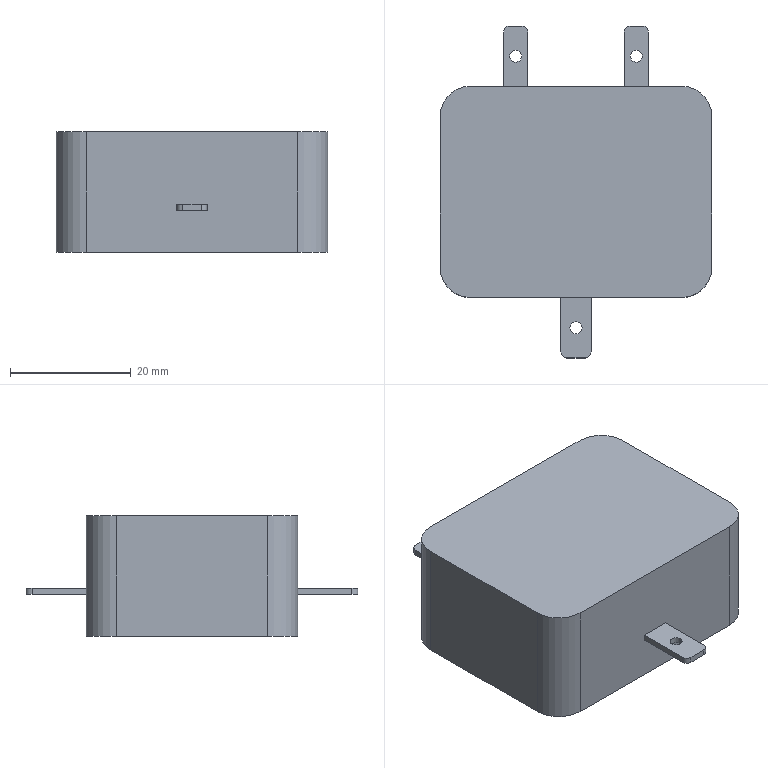Part | SolidWorks | features ICE 2, Extrusion 1 | 1 solid | 37 faces | box 45 x 55 x 20 mm | volume 31190 mm3 | plane 21 | cylinder 16 | commonest cylinder face diameters 2 x12 10 x4
STEP:
#1=CARTESIAN_POINT('',(11.,22.5,-2.));
#2=VERTEX_POINT('',#1);
#3=CARTESIAN_POINT('',(9.,22.5,-2.));
#4=VERTEX_POINT('',#3);
#5=CARTESIAN_POINT('',(10.,22.5,-2.));
#6=DIRECTION('',(0.,0.,-1.));
#7=DIRECTION('',(-1.,0.,0.));
#8=AXIS2_PLACEMENT_3D('',#5,#6,#7);
#9=CIRCLE('',#8,1.);
#10=EDGE_CURVE('',#2,#4,#9,.T.);
#11=ORIENTED_EDGE('',*,*,#10,.F.);
#12=CARTESIAN_POINT('',(11.,22.5,-3.));
#13=VERTEX_POINT('',#12);
#14=CARTESIAN_POINT('',(11.,22.5,-2.));
#15=DIRECTION('',(0.,0.,-1.));
#16=VECTOR('',#15,1000.);
#17=LINE('',#14,#16);
#18=EDGE_CURVE('',#2,#13,#17,.T.);
#19=ORIENTED_EDGE('',*,*,#18,.T.);
#20=CARTESIAN_POINT('',(9.,22.5,-3.));
#21=VERTEX_POINT('',#20);
#22=CARTESIAN_POINT('',(10.,22.5,-3.));
#23=DIRECTION('',(0.,0.,-1.));
#24=DIRECTION('',(-1.,0.,0.));
#25=AXIS2_PLACEMENT_3D('',#22,#23,#24);
#26=CIRCLE('',#25,1.);
#27=EDGE_CURVE('',#13,#21,#26,.T.);
#28=ORIENTED_EDGE('',*,*,#27,.T.);
#29=CARTESIAN_POINT('',(9.,22.5,-2.));
#30=DIRECTION('',(0.,0.,-1.));
#31=VECTOR('',#30,1000.);
#32=LINE('',#29,#31);
#33=EDGE_CURVE('',#4,#21,#32,.T.);
#34=ORIENTED_EDGE('',*,*,#33,.F.);
#35=EDGE_LOOP('',(#11,#19,#28,#34));
#36=FACE_OUTER_BOUND('',#35,.T.);
#37=CARTESIAN_POINT('',(10.,22.5,-2.));
#38=DIRECTION('',(0.,0.,-1.));
#39=DIRECTION('',(-1.,0.,0.));
#40=AXIS2_PLACEMENT_3D('',#37,#38,#39);
#41=CYLINDRICAL_SURFACE('',#40,1.);
#42=ADVANCED_FACE('',(#36),#41,.F.);
#43=CARTESIAN_POINT('',(-9.,22.5,-2.));
#44=VERTEX_POINT('',#43);
#45=CARTESIAN_POINT('',(-11.,22.5,-2.));
#46=VERTEX_POINT('',#45);
#47=CARTESIAN_POINT('',(-10.,22.5,-2.));
#48=DIRECTION('',(0.,0.,-1.));
#49=DIRECTION('',(-1.,0.,0.));
#50=AXIS2_PLACEMENT_3D('',#47,#48,#49);
#51=CIRCLE('',#50,1.);
#52=EDGE_CURVE('',#44,#46,#51,.T.);
#53=ORIENTED_EDGE('',*,*,#52,.F.);
#54=CARTESIAN_POINT('',(-9.,22.5,-3.));
#55=VERTEX_POINT('',#54);
#56=CARTESIAN_POINT('',(-9.,22.5,-2.));
#57=DIRECTION('',(0.,0.,-1.));
#58=VECTOR('',#57,1000.);
#59=LINE('',#56,#58);
#60=EDGE_CURVE('',#44,#55,#59,.T.);
#61=ORIENTED_EDGE('',*,*,#60,.T.);
#62=CARTESIAN_POINT('',(-11.,22.5,-3.));
#63=VERTEX_POINT('',#62);
#64=CARTESIAN_POINT('',(-10.,22.5,-3.));
#65=DIRECTION('',(0.,0.,-1.));
#66=DIRECTION('',(-1.,0.,0.));
#67=AXIS2_PLACEMENT_3D('',#64,#65,#66);
#68=CIRCLE('',#67,1.);
#69=EDGE_CURVE('',#55,#63,#68,.T.);
#70=ORIENTED_EDGE('',*,*,#69,.T.);
#71=CARTESIAN_POINT('',(-11.,22.5,-2.));
#72=DIRECTION('',(0.,0.,-1.));
#73=VECTOR('',#72,1000.);
#74=LINE('',#71,#73);
#75=EDGE_CURVE('',#46,#63,#74,.T.);
#76=ORIENTED_EDGE('',*,*,#75,.F.);
#77=EDGE_LOOP('',(#53,#61,#70,#76));
#78=FACE_OUTER_BOUND('',#77,.T.);
#79=CARTESIAN_POINT('',(-10.,22.5,-2.));
#80=DIRECTION('',(0.,0.,-1.));
#81=DIRECTION('',(-1.,0.,0.));
#82=AXIS2_PLACEMENT_3D('',#79,#80,#81);
#83=CYLINDRICAL_SURFACE('',#82,1.);
#84=ADVANCED_FACE('',(#78),#83,.F.);
#85=CARTESIAN_POINT('',(1.,-22.5,-2.));
#86=VERTEX_POINT('',#85);
#87=CARTESIAN_POINT('',(-1.,-22.5,-2.));
#88=VERTEX_POINT('',#87);
#89=CARTESIAN_POINT('',(0.,-22.5,-2.));
#90=DIRECTION('',(0.,0.,-1.));
#91=DIRECTION('',(-1.,0.,0.));
#92=AXIS2_PLACEMENT_3D('',#89,#90,#91);
#93=CIRCLE('',#92,1.);
#94=EDGE_CURVE('',#86,#88,#93,.T.);
#95=ORIENTED_EDGE('',*,*,#94,.F.);
#96=CARTESIAN_POINT('',(1.,-22.5,-3.));
#97=VERTEX_POINT('',#96);
#98=CARTESIAN_POINT('',(1.,-22.5,-2.));
#99=DIRECTION('',(0.,0.,-1.));
#100=VECTOR('',#99,1000.);
#101=LINE('',#98,#100);
#102=EDGE_CURVE('',#86,#97,#101,.T.);
#103=ORIENTED_EDGE('',*,*,#102,.T.);
#104=CARTESIAN_POINT('',(-1.,-22.5,-3.));
#105=VERTEX_POINT('',#104);
#106=CARTESIAN_POINT('',(0.,-22.5,-3.));
#107=DIRECTION('',(0.,0.,-1.));
#108=DIRECTION('',(-1.,0.,0.));
#109=AXIS2_PLACEMENT_3D('',#106,#107,#108);
#110=CIRCLE('',#109,1.);
#111=EDGE_CURVE('',#97,#105,#110,.T.);
#112=ORIENTED_EDGE('',*,*,#111,.T.);
#113=CARTESIAN_POINT('',(-1.,-22.5,-2.));
#114=DIRECTION('',(0.,0.,-1.));
#115=VECTOR('',#114,1000.);
#116=LINE('',#113,#115);
#117=EDGE_CURVE('',#88,#105,#116,.T.);
#118=ORIENTED_EDGE('',*,*,#117,.F.);
#119=EDGE_LOOP('',(#95,#103,#112,#118));
#120=FACE_OUTER_BOUND('',#119,.T.);
#121=CARTESIAN_POINT('',(0.,-22.5,-2.));
#122=DIRECTION('',(0.,0.,-1.));
#123=DIRECTION('',(-1.,0.,0.));
#124=AXIS2_PLACEMENT_3D('',#121,#122,#123);
#125=CYLINDRICAL_SURFACE('',#124,1.);
#126=ADVANCED_FACE('',(#120),#125,.F.);
#127=CARTESIAN_POINT('',(-17.5,-17.5,-10.));
#128=VERTEX_POINT('',#127);
#129=CARTESIAN_POINT('',(17.5,-17.5,-10.));
#130=VERTEX_POINT('',#129);
#131=CARTESIAN_POINT('',(-17.5,-17.5,-10.));
#132=DIRECTION('',(1.,0.,0.));
#133=VECTOR('',#132,1000.);
#134=LINE('',#131,#133);
#135=EDGE_CURVE('',#128,#130,#134,.T.);
#136=ORIENTED_EDGE('',*,*,#135,.T.);
#137=CARTESIAN_POINT('',(17.5,-17.5,10.));
#138=VERTEX_POINT('',#137);
#139=CARTESIAN_POINT('',(17.5,-17.5,10.));
#140=DIRECTION('',(0.,0.,-1.));
#141=VECTOR('',#140,1000.);
#142=LINE('',#139,#141);
#143=EDGE_CURVE('',#138,#130,#142,.T.);
#144=ORIENTED_EDGE('',*,*,#143,.F.);
#145=CARTESIAN_POINT('',(-17.5,-17.5,10.));
#146=VERTEX_POINT('',#145);
#147=CARTESIAN_POINT('',(-17.5,-17.5,10.));
#148=DIRECTION('',(1.,0.,0.));
#149=VECTOR('',#148,1000.);
#150=LINE('',#147,#149);
#151=EDGE_CURVE('',#146,#138,#150,.T.);
#152=ORIENTED_EDGE('',*,*,#151,.F.);
#153=CARTESIAN_POINT('',(-17.5,-17.5,10.));
#154=DIRECTION('',(0.,0.,-1.));
#155=VECTOR('',#154,1000.);
#156=LINE('',#153,#155);
#157=EDGE_CURVE('',#146,#128,#156,.T.);
#158=ORIENTED_EDGE('',*,*,#157,.T.);
#159=EDGE_LOOP('',(#136,#144,#152,#158));
#160=FACE_OUTER_BOUND('',#159,.T.);
#161=CARTESIAN_POINT('',(-2.5,-17.5,-2.));
#162=VERTEX_POINT('',#161);
#163=CARTESIAN_POINT('',(2.5,-17.5,-2.));
#164=VERTEX_POINT('',#163);
#165=CARTESIAN_POINT('',(2.5,-17.5,-2.));
#166=DIRECTION('',(1.,0.,0.));
#167=VECTOR('',#166,1000.);
#168=LINE('',#165,#167);
#169=EDGE_CURVE('',#162,#164,#168,.T.);
#170=ORIENTED_EDGE('',*,*,#169,.T.);
#171=CARTESIAN_POINT('',(2.5,-17.5,-3.));
#172=VERTEX_POINT('',#171);
#173=CARTESIAN_POINT('',(2.5,-17.5,-2.));
#174=DIRECTION('',(0.,0.,-1.));
#175=VECTOR('',#174,1000.);
#176=LINE('',#173,#175);
#177=EDGE_CURVE('',#164,#172,#176,.T.);
#178=ORIENTED_EDGE('',*,*,#177,.T.);
#179=CARTESIAN_POINT('',(-2.5,-17.5,-3.));
#180=VERTEX_POINT('',#179);
#181=CARTESIAN_POINT('',(2.5,-17.5,-3.));
#182=DIRECTION('',(1.,0.,0.));
#183=VECTOR('',#182,1000.);
#184=LINE('',#181,#183);
#185=EDGE_CURVE('',#180,#172,#184,.T.);
#186=ORIENTED_EDGE('',*,*,#185,.F.);
#187=CARTESIAN_POINT('',(-2.5,-17.5,-2.));
#188=DIRECTION('',(0.,0.,-1.));
#189=VECTOR('',#188,1000.);
#190=LINE('',#187,#189);
#191=EDGE_CURVE('',#162,#180,#190,.T.);
#192=ORIENTED_EDGE('',*,*,#191,.F.);
#193=EDGE_LOOP('',(#170,#178,#186,#192));
#194=FACE_BOUND('',#193,.T.);
#195=CARTESIAN_POINT('',(-17.5,-17.5,10.));
#196=DIRECTION('',(0.,1.,0.));
#197=DIRECTION('',(0.,0.,1.));
#198=AXIS2_PLACEMENT_3D('',#195,#196,#197);
#199=PLANE('',#198);
#200=ADVANCED_FACE('',(#160,#194),#199,.F.);
#201=CARTESIAN_POINT('',(-8.,17.5,-2.));
#202=VERTEX_POINT('',#201);
#203=CARTESIAN_POINT('',(-8.,17.5,-3.));
#204=VERTEX_POINT('',#203);
#205=CARTESIAN_POINT('',(-8.,17.5,-2.));
#206=DIRECTION('',(0.,0.,-1.));
#207=VECTOR('',#206,1000.);
#208=LINE('',#205,#207);
#209=EDGE_CURVE('',#202,#204,#208,.T.);
#210=ORIENTED_EDGE('',*,*,#209,.F.);
#211=CARTESIAN_POINT('',(-12.,17.5,-2.));
#212=VERTEX_POINT('',#211);
#213=CARTESIAN_POINT('',(-8.,17.5,-2.));
#214=DIRECTION('',(-1.,0.,0.));
#215=VECTOR('',#214,1000.);
#216=LINE('',#213,#215);
#217=EDGE_CURVE('',#202,#212,#216,.T.);
#218=ORIENTED_EDGE('',*,*,#217,.T.);
#219=CARTESIAN_POINT('',(-12.,17.5,-3.));
#220=VERTEX_POINT('',#219);
#221=CARTESIAN_POINT('',(-12.,17.5,-2.));
#222=DIRECTION('',(0.,0.,-1.));
#223=VECTOR('',#222,1000.);
#224=LINE('',#221,#223);
#225=EDGE_CURVE('',#212,#220,#224,.T.);
#226=ORIENTED_EDGE('',*,*,#225,.T.);
#227=CARTESIAN_POINT('',(-8.,17.5,-3.));
#228=DIRECTION('',(-1.,0.,0.));
#229=VECTOR('',#228,1000.);
#230=LINE('',#227,#229);
#231=EDGE_CURVE('',#204,#220,#230,.T.);
#232=ORIENTED_EDGE('',*,*,#231,.F.);
#233=EDGE_LOOP('',(#210,#218,#226,#232));
#234=FACE_BOUND('',#233,.T.);
#235=CARTESIAN_POINT('',(17.5,17.5,-10.));
#236=VERTEX_POINT('',#235);
#237=CARTESIAN_POINT('',(-17.5,17.5,-10.));
#238=VERTEX_POINT('',#237);
#239=CARTESIAN_POINT('',(-17.5,17.5,-10.));
#240=DIRECTION('',(-1.,0.,0.));
#241=VECTOR('',#240,1000.);
#242=LINE('',#239,#241);
#243=EDGE_CURVE('',#236,#238,#242,.T.);
#244=ORIENTED_EDGE('',*,*,#243,.T.);
#245=CARTESIAN_POINT('',(-17.5,17.5,10.));
#246=VERTEX_POINT('',#245);
#247=CARTESIAN_POINT('',(-17.5,17.5,10.));
#248=DIRECTION('',(0.,0.,-1.));
#249=VECTOR('',#248,1000.);
#250=LINE('',#247,#249);
#251=EDGE_CURVE('',#246,#238,#250,.T.);
#252=ORIENTED_EDGE('',*,*,#251,.F.);
#253=CARTESIAN_POINT('',(17.5,17.5,10.));
#254=VERTEX_POINT('',#253);
#255=CARTESIAN_POINT('',(-17.5,17.5,10.));
#256=DIRECTION('',(-1.,0.,0.));
#257=VECTOR('',#256,1000.);
#258=LINE('',#255,#257);
#259=EDGE_CURVE('',#254,#246,#258,.T.);
#260=ORIENTED_EDGE('',*,*,#259,.F.);
#261=CARTESIAN_POINT('',(17.5,17.5,10.));
#262=DIRECTION('',(0.,0.,-1.));
#263=VECTOR('',#262,1000.);
#264=LINE('',#261,#263);
#265=EDGE_CURVE('',#254,#236,#264,.T.);
#266=ORIENTED_EDGE('',*,*,#265,.T.);
#267=EDGE_LOOP('',(#244,#252,#260,#266));
#268=FACE_OUTER_BOUND('',#267,.T.);
#269=CARTESIAN_POINT('',(12.,17.5,-2.));
#270=VERTEX_POINT('',#269);
#271=CARTESIAN_POINT('',(8.,17.5,-2.));
#272=VERTEX_POINT('',#271);
#273=CARTESIAN_POINT('',(8.,17.5,-2.));
#274=DIRECTION('',(-1.,0.,0.));
#275=VECTOR('',#274,1000.);
#276=LINE('',#273,#275);
#277=EDGE_CURVE('',#270,#272,#276,.T.);
#278=ORIENTED_EDGE('',*,*,#277,.T.);
#279=CARTESIAN_POINT('',(8.,17.5,-3.));
#280=VERTEX_POINT('',#279);
#281=CARTESIAN_POINT('',(8.,17.5,-2.));
#282=DIRECTION('',(0.,0.,-1.));
#283=VECTOR('',#282,1000.);
#284=LINE('',#281,#283);
#285=EDGE_CURVE('',#272,#280,#284,.T.);
#286=ORIENTED_EDGE('',*,*,#285,.T.);
#287=CARTESIAN_POINT('',(12.,17.5,-3.));
#288=VERTEX_POINT('',#287);
#289=CARTESIAN_POINT('',(8.,17.5,-3.));
#290=DIRECTION('',(-1.,0.,0.));
#291=VECTOR('',#290,1000.);
#292=LINE('',#289,#291);
#293=EDGE_CURVE('',#288,#280,#292,.T.);
#294=ORIENTED_EDGE('',*,*,#293,.F.);
#295=CARTESIAN_POINT('',(12.,17.5,-2.));
#296=DIRECTION('',(0.,0.,-1.));
#297=VECTOR('',#296,1000.);
#298=LINE('',#295,#297);
#299=EDGE_CURVE('',#270,#288,#298,.T.);
#300=ORIENTED_EDGE('',*,*,#299,.F.);
#301=EDGE_LOOP('',(#278,#286,#294,#300));
#302=FACE_BOUND('',#301,.T.);
#303=CARTESIAN_POINT('',(-17.5,17.5,10.));
#304=DIRECTION('',(0.,-1.,0.));
#305=DIRECTION('',(0.,0.,-1.));
#306=AXIS2_PLACEMENT_3D('',#303,#304,#305);
#307=PLANE('',#306);
#308=ADVANCED_FACE('',(#234,#268,#302),#307,.F.);
#309=CARTESIAN_POINT('',(-22.5,-12.5,-10.));
#310=VERTEX_POINT('',#309);
#311=CARTESIAN_POINT('',(-17.5,-12.5,-10.));
#312=DIRECTION('',(0.,0.,1.));
#313=DIRECTION('',(-1.,0.,0.));
#314=AXIS2_PLACEMENT_3D('',#311,#312,#313);
#315=CIRCLE('',#314,5.);
#316=EDGE_CURVE('',#310,#128,#315,.T.);
#317=ORIENTED_EDGE('',*,*,#316,.T.);
#318=ORIENTED_EDGE('',*,*,#157,.F.);
#319=CARTESIAN_POINT('',(-22.5,-12.5,10.));
#320=VERTEX_POINT('',#319);
#321=CARTESIAN_POINT('',(-17.5,-12.5,10.));
#322=DIRECTION('',(0.,0.,1.));
#323=DIRECTION('',(-1.,0.,0.));
#324=AXIS2_PLACEMENT_3D('',#321,#322,#323);
#325=CIRCLE('',#324,5.);
#326=EDGE_CURVE('',#320,#146,#325,.T.);
#327=ORIENTED_EDGE('',*,*,#326,.F.);
#328=CARTESIAN_POINT('',(-22.5,-12.5,10.));
#329=DIRECTION('',(0.,0.,-1.));
#330=VECTOR('',#329,1000.);
#331=LINE('',#328,#330);
#332=EDGE_CURVE('',#320,#310,#331,.T.);
#333=ORIENTED_EDGE('',*,*,#332,.T.);
#334=EDGE_LOOP('',(#317,#318,#327,#333));
#335=FACE_OUTER_BOUND('',#334,.T.);
#336=CARTESIAN_POINT('',(-17.5,-12.5,10.));
#337=DIRECTION('',(0.,0.,-1.));
#338=DIRECTION('',(-1.,0.,0.));
#339=AXIS2_PLACEMENT_3D('',#336,#337,#338);
#340=CYLINDRICAL_SURFACE('',#339,5.);
#341=ADVANCED_FACE('',(#335),#340,.T.);
#342=CARTESIAN_POINT('',(22.5,-12.5,-10.));
#343=VERTEX_POINT('',#342);
#344=CARTESIAN_POINT('',(17.5,-12.5,-10.));
#345=DIRECTION('',(0.,0.,1.));
#346=DIRECTION('',(1.,0.,0.));
#347=AXIS2_PLACEMENT_3D('',#344,#345,#346);
#348=CIRCLE('',#347,5.);
#349=EDGE_CURVE('',#130,#343,#348,.T.);
#350=ORIENTED_EDGE('',*,*,#349,.T.);
#351=CARTESIAN_POINT('',(22.5,-12.5,10.));
#352=VERTEX_POINT('',#351);
#353=CARTESIAN_POINT('',(22.5,-12.5,10.));
#354=DIRECTION('',(0.,0.,-1.));
#355=VECTOR('',#354,1000.);
#356=LINE('',#353,#355);
#357=EDGE_CURVE('',#352,#343,#356,.T.);
#358=ORIENTED_EDGE('',*,*,#357,.F.);
#359=CARTESIAN_POINT('',(17.5,-12.5,10.));
#360=DIRECTION('',(0.,0.,1.));
#361=DIRECTION('',(1.,0.,0.));
#362=AXIS2_PLACEMENT_3D('',#359,#360,#361);
#363=CIRCLE('',#362,5.);
#364=EDGE_CURVE('',#138,#352,#363,.T.);
#365=ORIENTED_EDGE('',*,*,#364,.F.);
#366=ORIENTED_EDGE('',*,*,#143,.T.);
#367=EDGE_LOOP('',(#350,#358,#365,#366));
#368=FACE_OUTER_BOUND('',#367,.T.);
#369=CARTESIAN_POINT('',(17.5,-12.5,10.));
#370=DIRECTION('',(0.,0.,-1.));
#371=DIRECTION('',(-1.,0.,0.));
#372=AXIS2_PLACEMENT_3D('',#369,#370,#371);
#373=CYLINDRICAL_SURFACE('',#372,5.);
#374=ADVANCED_FACE('',(#368),#373,.T.);
#375=CARTESIAN_POINT('',(22.5,12.5,-10.));
#376=VERTEX_POINT('',#375);
#377=CARTESIAN_POINT('',(22.5,-12.5,-10.));
#378=DIRECTION('',(0.,1.,0.));
#379=VECTOR('',#378,1000.);
#380=LINE('',#377,#379);
#381=EDGE_CURVE('',#343,#376,#380,.T.);
#382=ORIENTED_EDGE('',*,*,#381,.T.);
#383=CARTESIAN_POINT('',(22.5,12.5,10.));
#384=VERTEX_POINT('',#383);
#385=CARTESIAN_POINT('',(22.5,12.5,10.));
#386=DIRECTION('',(0.,0.,-1.));
#387=VECTOR('',#386,1000.);
#388=LINE('',#385,#387);
#389=EDGE_CURVE('',#384,#376,#388,.T.);
#390=ORIENTED_EDGE('',*,*,#389,.F.);
#391=CARTESIAN_POINT('',(22.5,-12.5,10.));
#392=DIRECTION('',(0.,1.,0.));
#393=VECTOR('',#392,1000.);
#394=LINE('',#391,#393);
#395=EDGE_CURVE('',#352,#384,#394,.T.);
#396=ORIENTED_EDGE('',*,*,#395,.F.);
#397=ORIENTED_EDGE('',*,*,#357,.T.);
#398=EDGE_LOOP('',(#382,#390,#396,#397));
#399=FACE_OUTER_BOUND('',#398,.T.);
#400=CARTESIAN_POINT('',(22.5,-12.5,10.));
#401=DIRECTION('',(-1.,0.,0.));
#402=DIRECTION('',(0.,0.,1.));
#403=AXIS2_PLACEMENT_3D('',#400,#401,#402);
#404=PLANE('',#403);
#405=ADVANCED_FACE('',(#399),#404,.F.);
#406=CARTESIAN_POINT('',(17.5,12.5,-10.));
#407=DIRECTION('',(0.,0.,1.));
#408=DIRECTION('',(-1.,0.,0.));
#409=AXIS2_PLACEMENT_3D('',#406,#407,#408);
#410=CIRCLE('',#409,5.);
#411=EDGE_CURVE('',#376,#236,#410,.T.);
#412=ORIENTED_EDGE('',*,*,#411,.T.);
#413=ORIENTED_EDGE('',*,*,#265,.F.);
#414=CARTESIAN_POINT('',(17.5,12.5,10.));
#415=DIRECTION('',(0.,0.,1.));
#416=DIRECTION('',(-1.,0.,0.));
#417=AXIS2_PLACEMENT_3D('',#414,#415,#416);
#418=CIRCLE('',#417,5.);
#419=EDGE_CURVE('',#384,#254,#418,.T.);
#420=ORIENTED_EDGE('',*,*,#419,.F.);
#421=ORIENTED_EDGE('',*,*,#389,.T.);
#422=EDGE_LOOP('',(#412,#413,#420,#421));
#423=FACE_OUTER_BOUND('',#422,.T.);
#424=CARTESIAN_POINT('',(17.5,12.5,10.));
#425=DIRECTION('',(0.,0.,-1.));
#426=DIRECTION('',(-1.,0.,0.));
#427=AXIS2_PLACEMENT_3D('',#424,#425,#426);
#428=CYLINDRICAL_SURFACE('',#427,5.);
#429=ADVANCED_FACE('',(#423),#428,.T.);
#430=CARTESIAN_POINT('',(-22.5,12.5,-10.));
#431=VERTEX_POINT('',#430);
#432=CARTESIAN_POINT('',(-17.5,12.5,-10.));
#433=DIRECTION('',(0.,0.,1.));
#434=DIRECTION('',(-1.,0.,0.));
#435=AXIS2_PLACEMENT_3D('',#432,#433,#434);
#436=CIRCLE('',#435,5.);
#437=EDGE_CURVE('',#238,#431,#436,.T.);
#438=ORIENTED_EDGE('',*,*,#437,.T.);
#439=CARTESIAN_POINT('',(-22.5,12.5,10.));
#440=VERTEX_POINT('',#439);
#441=CARTESIAN_POINT('',(-22.5,12.5,10.));
#442=DIRECTION('',(0.,0.,-1.));
#443=VECTOR('',#442,1000.);
#444=LINE('',#441,#443);
#445=EDGE_CURVE('',#440,#431,#444,.T.);
#446=ORIENTED_EDGE('',*,*,#445,.F.);
#447=CARTESIAN_POINT('',(-17.5,12.5,10.));
#448=DIRECTION('',(0.,0.,1.));
#449=DIRECTION('',(-1.,0.,0.));
#450=AXIS2_PLACEMENT_3D('',#447,#448,#449);
#451=CIRCLE('',#450,5.);
#452=EDGE_CURVE('',#246,#440,#451,.T.);
#453=ORIENTED_EDGE('',*,*,#452,.F.);
#454=ORIENTED_EDGE('',*,*,#251,.T.);
#455=EDGE_LOOP('',(#438,#446,#453,#454));
#456=FACE_OUTER_BOUND('',#455,.T.);
#457=CARTESIAN_POINT('',(-17.5,12.5,10.));
#458=DIRECTION('',(0.,0.,-1.));
#459=DIRECTION('',(-1.,0.,0.));
#460=AXIS2_PLACEMENT_3D('',#457,#458,#459);
#461=CYLINDRICAL_SURFACE('',#460,5.);
#462=ADVANCED_FACE('',(#456),#461,.T.);
#463=CARTESIAN_POINT('',(-22.5,-12.5,-10.));
#464=DIRECTION('',(0.,-1.,0.));
#465=VECTOR('',#464,1000.);
#466=LINE('',#463,#465);
#467=EDGE_CURVE('',#431,#310,#466,.T.);
#468=ORIENTED_EDGE('',*,*,#467,.T.);
#469=ORIENTED_EDGE('',*,*,#332,.F.);
#470=CARTESIAN_POINT('',(-22.5,-12.5,10.));
#471=DIRECTION('',(0.,-1.,0.));
#472=VECTOR('',#471,1000.);
#473=LINE('',#470,#472);
#474=EDGE_CURVE('',#440,#320,#473,.T.);
#475=ORIENTED_EDGE('',*,*,#474,.F.);
#476=ORIENTED_EDGE('',*,*,#445,.T.);
#477=EDGE_LOOP('',(#468,#469,#475,#476));
#478=FACE_OUTER_BOUND('',#477,.T.);
#479=CARTESIAN_POINT('',(-22.5,-12.5,10.));
#480=DIRECTION('',(1.,0.,0.));
#481=DIRECTION('',(0.,0.,-1.));
#482=AXIS2_PLACEMENT_3D('',#479,#480,#481);
#483=PLANE('',#482);
#484=ADVANCED_FACE('',(#478),#483,.F.);
#485=ORIENTED_EDGE('',*,*,#326,.T.);
#486=ORIENTED_EDGE('',*,*,#151,.T.);
#487=ORIENTED_EDGE('',*,*,#364,.T.);
#488=ORIENTED_EDGE('',*,*,#395,.T.);
#489=ORIENTED_EDGE('',*,*,#419,.T.);
#490=ORIENTED_EDGE('',*,*,#259,.T.);
#491=ORIENTED_EDGE('',*,*,#452,.T.);
#492=ORIENTED_EDGE('',*,*,#474,.T.);
#493=EDGE_LOOP('',(#485,#486,#487,#488,#489,#490,#491,#492));
#494=FACE_OUTER_BOUND('',#493,.T.);
#495=CARTESIAN_POINT('',(-17.5,-12.5,10.));
#496=DIRECTION('',(0.,0.,-1.));
#497=DIRECTION('',(-1.,0.,0.));
#498=AXIS2_PLACEMENT_3D('',#495,#496,#497);
#499=PLANE('',#498);
#500=ADVANCED_FACE('',(#494),#499,.F.);
#501=ORIENTED_EDGE('',*,*,#316,.F.);
#502=ORIENTED_EDGE('',*,*,#467,.F.);
#503=ORIENTED_EDGE('',*,*,#437,.F.);
#504=ORIENTED_EDGE('',*,*,#243,.F.);
#505=ORIENTED_EDGE('',*,*,#411,.F.);
#506=ORIENTED_EDGE('',*,*,#381,.F.);
#507=ORIENTED_EDGE('',*,*,#349,.F.);
#508=ORIENTED_EDGE('',*,*,#135,.F.);
#509=EDGE_LOOP('',(#501,#502,#503,#504,#505,#506,#507,#508));
#510=FACE_OUTER_BOUND('',#509,.T.);
#511=CARTESIAN_POINT('',(-17.5,-12.5,-10.));
#512=DIRECTION('',(0.,0.,-1.));
#513=DIRECTION('',(-1.,0.,0.));
#514=AXIS2_PLACEMENT_3D('',#511,#512,#513);
#515=PLANE('',#514);
#516=ADVANCED_FACE('',(#510),#515,.T.);
#517=CARTESIAN_POINT('',(8.,26.5,-3.));
#518=VERTEX_POINT('',#517);
#519=CARTESIAN_POINT('',(8.,17.5,-3.));
#520=DIRECTION('',(0.,1.,0.));
#521=VECTOR('',#520,1000.);
#522=LINE('',#519,#521);
#523=EDGE_CURVE('',#280,#518,#522,.T.);
#524=ORIENTED_EDGE('',*,*,#523,.F.);
#525=ORIENTED_EDGE('',*,*,#285,.F.);
#526=CARTESIAN_POINT('',(8.,26.5,-2.));
#527=VERTEX_POINT('',#526);
#528=CARTESIAN_POINT('',(8.,17.5,-2.));
#529=DIRECTION('',(0.,1.,0.));
#530=VECTOR('',#529,1000.);
#531=LINE('',#528,#530);
#532=EDGE_CURVE('',#272,#527,#531,.T.);
#533=ORIENTED_EDGE('',*,*,#532,.T.);
#534=CARTESIAN_POINT('',(8.,26.5,-2.));
#535=DIRECTION('',(0.,0.,-1.));
#536=VECTOR('',#535,1000.);
#537=LINE('',#534,#536);
#538=EDGE_CURVE('',#527,#518,#537,.T.);
#539=ORIENTED_EDGE('',*,*,#538,.T.);
#540=EDGE_LOOP('',(#524,#525,#533,#539));
#541=FACE_OUTER_BOUND('',#540,.T.);
#542=CARTESIAN_POINT('',(8.,17.5,-2.));
#543=DIRECTION('',(-1.,0.,0.));
#544=DIRECTION('',(0.,-1.,0.));
#545=AXIS2_PLACEMENT_3D('',#542,#543,#544);
#546=PLANE('',#545);
#547=ADVANCED_FACE('',(#541),#546,.T.);
#548=CARTESIAN_POINT('',(12.,26.5,-3.));
#549=VERTEX_POINT('',#548);
#550=CARTESIAN_POINT('',(12.,17.5,-3.));
#551=DIRECTION('',(0.,-1.,0.));
#552=VECTOR('',#551,1000.);
#553=LINE('',#550,#552);
#554=EDGE_CURVE('',#549,#288,#553,.T.);
#555=ORIENTED_EDGE('',*,*,#554,.F.);
#556=CARTESIAN_POINT('',(12.,26.5,-2.));
#557=VERTEX_POINT('',#556);
#558=CARTESIAN_POINT('',(12.,26.5,-2.));
#559=DIRECTION('',(0.,0.,-1.));
#560=VECTOR('',#559,1000.);
#561=LINE('',#558,#560);
#562=EDGE_CURVE('',#557,#549,#561,.T.);
#563=ORIENTED_EDGE('',*,*,#562,.F.);
#564=CARTESIAN_POINT('',(12.,17.5,-2.));
#565=DIRECTION('',(0.,-1.,0.));
#566=VECTOR('',#565,1000.);
#567=LINE('',#564,#566);
#568=EDGE_CURVE('',#557,#270,#567,.T.);
#569=ORIENTED_EDGE('',*,*,#568,.T.);
#570=ORIENTED_EDGE('',*,*,#299,.T.);
#571=EDGE_LOOP('',(#555,#563,#569,#570));
#572=FACE_OUTER_BOUND('',#571,.T.);
#573=CARTESIAN_POINT('',(12.,17.5,-2.));
#574=DIRECTION('',(1.,0.,0.));
#575=DIRECTION('',(0.,0.,-1.));
#576=AXIS2_PLACEMENT_3D('',#573,#574,#575);
#577=PLANE('',#576);
#578=ADVANCED_FACE('',(#572),#577,.T.);
#579=CARTESIAN_POINT('',(11.,27.5,-3.));
#580=VERTEX_POINT('',#579);
#581=CARTESIAN_POINT('',(11.,26.5,-3.));
#582=DIRECTION('',(0.,0.,-1.));
#583=DIRECTION('',(-1.,0.,0.));
#584=AXIS2_PLACEMENT_3D('',#581,#582,#583);
#585=CIRCLE('',#584,1.);
#586=EDGE_CURVE('',#580,#549,#585,.T.);
#587=ORIENTED_EDGE('',*,*,#586,.F.);
#588=CARTESIAN_POINT('',(11.,27.5,-2.));
#589=VERTEX_POINT('',#588);
#590=CARTESIAN_POINT('',(11.,27.5,-2.));
#591=DIRECTION('',(0.,0.,-1.));
#592=VECTOR('',#591,1000.);
#593=LINE('',#590,#592);
#594=EDGE_CURVE('',#589,#580,#593,.T.);
#595=ORIENTED_EDGE('',*,*,#594,.F.);
#596=CARTESIAN_POINT('',(11.,26.5,-2.));
#597=DIRECTION('',(0.,0.,-1.));
#598=DIRECTION('',(-1.,0.,0.));
#599=AXIS2_PLACEMENT_3D('',#596,#597,#598);
#600=CIRCLE('',#599,1.);
#601=EDGE_CURVE('',#589,#557,#600,.T.);
#602=ORIENTED_EDGE('',*,*,#601,.T.);
#603=ORIENTED_EDGE('',*,*,#562,.T.);
#604=EDGE_LOOP('',(#587,#595,#602,#603));
#605=FACE_OUTER_BOUND('',#604,.T.);
#606=CARTESIAN_POINT('',(11.,26.5,-2.));
#607=DIRECTION('',(0.,0.,-1.));
#608=DIRECTION('',(-1.,0.,0.));
#609=AXIS2_PLACEMENT_3D('',#606,#607,#608);
#610=CYLINDRICAL_SURFACE('',#609,1.);
#611=ADVANCED_FACE('',(#605),#610,.T.);
#612=CARTESIAN_POINT('',(9.,27.5,-3.));
#613=VERTEX_POINT('',#612);
#614=CARTESIAN_POINT('',(9.,27.5,-3.));
#615=DIRECTION('',(1.,0.,0.));
#616=VECTOR('',#615,1000.);
#617=LINE('',#614,#616);
#618=EDGE_CURVE('',#613,#580,#617,.T.);
#619=ORIENTED_EDGE('',*,*,#618,.F.);
#620=CARTESIAN_POINT('',(9.,27.5,-2.));
#621=VERTEX_POINT('',#620);
#622=CARTESIAN_POINT('',(9.,27.5,-2.));
#623=DIRECTION('',(0.,0.,-1.));
#624=VECTOR('',#623,1000.);
#625=LINE('',#622,#624);
#626=EDGE_CURVE('',#621,#613,#625,.T.);
#627=ORIENTED_EDGE('',*,*,#626,.F.);
#628=CARTESIAN_POINT('',(9.,27.5,-2.));
#629=DIRECTION('',(1.,0.,0.));
#630=VECTOR('',#629,1000.);
#631=LINE('',#628,#630);
#632=EDGE_CURVE('',#621,#589,#631,.T.);
#633=ORIENTED_EDGE('',*,*,#632,.T.);
#634=ORIENTED_EDGE('',*,*,#594,.T.);
#635=EDGE_LOOP('',(#619,#627,#633,#634));
#636=FACE_OUTER_BOUND('',#635,.T.);
#637=CARTESIAN_POINT('',(9.,27.5,-2.));
#638=DIRECTION('',(0.,1.,0.));
#639=DIRECTION('',(0.,0.,1.));
#640=AXIS2_PLACEMENT_3D('',#637,#638,#639);
#641=PLANE('',#640);
#642=ADVANCED_FACE('',(#636),#641,.T.);
#643=CARTESIAN_POINT('',(9.,26.5,-3.));
#644=DIRECTION('',(0.,0.,-1.));
#645=DIRECTION('',(-1.,0.,0.));
#646=AXIS2_PLACEMENT_3D('',#643,#644,#645);
#647=CIRCLE('',#646,1.);
#648=EDGE_CURVE('',#518,#613,#647,.T.);
#649=ORIENTED_EDGE('',*,*,#648,.F.);
#650=ORIENTED_EDGE('',*,*,#538,.F.);
#651=CARTESIAN_POINT('',(9.,26.5,-2.));
#652=DIRECTION('',(0.,0.,-1.));
#653=DIRECTION('',(-1.,0.,0.));
#654=AXIS2_PLACEMENT_3D('',#651,#652,#653);
#655=CIRCLE('',#654,1.);
#656=EDGE_CURVE('',#527,#621,#655,.T.);
#657=ORIENTED_EDGE('',*,*,#656,.T.);
#658=ORIENTED_EDGE('',*,*,#626,.T.);
#659=EDGE_LOOP('',(#649,#650,#657,#658));
#660=FACE_OUTER_BOUND('',#659,.T.);
#661=CARTESIAN_POINT('',(9.,26.5,-2.));
#662=DIRECTION('',(0.,0.,-1.));
#663=DIRECTION('',(-1.,0.,0.));
#664=AXIS2_PLACEMENT_3D('',#661,#662,#663);
#665=CYLINDRICAL_SURFACE('',#664,1.);
#666=ADVANCED_FACE('',(#660),#665,.T.);
#667=CARTESIAN_POINT('',(10.,22.5,-2.));
#668=DIRECTION('',(0.,0.,-1.));
#669=DIRECTION('',(-1.,0.,0.));
#670=AXIS2_PLACEMENT_3D('',#667,#668,#669);
#671=CIRCLE('',#670,1.);
#672=EDGE_CURVE('',#4,#2,#671,.T.);
#673=ORIENTED_EDGE('',*,*,#672,.T.);
#674=ORIENTED_EDGE('',*,*,#10,.T.);
#675=EDGE_LOOP('',(#673,#674));
#676=FACE_BOUND('',#675,.T.);
#677=ORIENTED_EDGE('',*,*,#532,.F.);
#678=ORIENTED_EDGE('',*,*,#277,.F.);
#679=ORIENTED_EDGE('',*,*,#568,.F.);
#680=ORIENTED_EDGE('',*,*,#601,.F.);
#681=ORIENTED_EDGE('',*,*,#632,.F.);
#682=ORIENTED_EDGE('',*,*,#656,.F.);
#683=EDGE_LOOP('',(#677,#678,#679,#680,#681,#682));
#684=FACE_OUTER_BOUND('',#683,.T.);
#685=CARTESIAN_POINT('',(9.,26.5,-2.));
#686=DIRECTION('',(0.,0.,-1.));
#687=DIRECTION('',(-1.,0.,0.));
#688=AXIS2_PLACEMENT_3D('',#685,#686,#687);
#689=PLANE('',#688);
#690=ADVANCED_FACE('',(#676,#684),#689,.F.);
#691=CARTESIAN_POINT('',(10.,22.5,-3.));
#692=DIRECTION('',(0.,0.,-1.));
#693=DIRECTION('',(-1.,0.,0.));
#694=AXIS2_PLACEMENT_3D('',#691,#692,#693);
#695=CIRCLE('',#694,1.);
#696=EDGE_CURVE('',#21,#13,#695,.T.);
#697=ORIENTED_EDGE('',*,*,#696,.F.);
#698=ORIENTED_EDGE('',*,*,#27,.F.);
#699=EDGE_LOOP('',(#697,#698));
#700=FACE_BOUND('',#699,.T.);
#701=ORIENTED_EDGE('',*,*,#523,.T.);
#702=ORIENTED_EDGE('',*,*,#648,.T.);
#703=ORIENTED_EDGE('',*,*,#618,.T.);
#704=ORIENTED_EDGE('',*,*,#586,.T.);
#705=ORIENTED_EDGE('',*,*,#554,.T.);
#706=ORIENTED_EDGE('',*,*,#293,.T.);
#707=EDGE_LOOP('',(#701,#702,#703,#704,#705,#706));
#708=FACE_OUTER_BOUND('',#707,.T.);
#709=CARTESIAN_POINT('',(9.,26.5,-3.));
#710=DIRECTION('',(0.,0.,-1.));
#711=DIRECTION('',(-1.,0.,0.));
#712=AXIS2_PLACEMENT_3D('',#709,#710,#711);
#713=PLANE('',#712);
#714=ADVANCED_FACE('',(#700,#708),#713,.T.);
#715=CARTESIAN_POINT('',(-8.,26.5,-3.));
#716=VERTEX_POINT('',#715);
#717=CARTESIAN_POINT('',(-8.,17.5,-3.));
#718=DIRECTION('',(0.,-1.,0.));
#719=VECTOR('',#718,1000.);
#720=LINE('',#717,#719);
#721=EDGE_CURVE('',#716,#204,#720,.T.);
#722=ORIENTED_EDGE('',*,*,#721,.F.);
#723=CARTESIAN_POINT('',(-8.,26.5,-2.));
#724=VERTEX_POINT('',#723);
#725=CARTESIAN_POINT('',(-8.,26.5,-2.));
#726=DIRECTION('',(0.,0.,-1.));
#727=VECTOR('',#726,1000.);
#728=LINE('',#725,#727);
#729=EDGE_CURVE('',#724,#716,#728,.T.);
#730=ORIENTED_EDGE('',*,*,#729,.F.);
#731=CARTESIAN_POINT('',(-8.,17.5,-2.));
#732=DIRECTION('',(0.,-1.,0.));
#733=VECTOR('',#732,1000.);
#734=LINE('',#731,#733);
#735=EDGE_CURVE('',#724,#202,#734,.T.);
#736=ORIENTED_EDGE('',*,*,#735,.T.);
#737=ORIENTED_EDGE('',*,*,#209,.T.);
#738=EDGE_LOOP('',(#722,#730,#736,#737));
#739=FACE_OUTER_BOUND('',#738,.T.);
#740=CARTESIAN_POINT('',(-8.,17.5,-2.));
#741=DIRECTION('',(1.,0.,0.));
#742=DIRECTION('',(0.,1.,0.));
#743=AXIS2_PLACEMENT_3D('',#740,#741,#742);
#744=PLANE('',#743);
#745=ADVANCED_FACE('',(#739),#744,.T.);
#746=CARTESIAN_POINT('',(-9.,27.5,-3.));
#747=VERTEX_POINT('',#746);
#748=CARTESIAN_POINT('',(-9.,26.5,-3.));
#749=DIRECTION('',(0.,0.,-1.));
#750=DIRECTION('',(1.,0.,0.));
#751=AXIS2_PLACEMENT_3D('',#748,#749,#750);
#752=CIRCLE('',#751,1.);
#753=EDGE_CURVE('',#747,#716,#752,.T.);
#754=ORIENTED_EDGE('',*,*,#753,.F.);
#755=CARTESIAN_POINT('',(-9.,27.5,-2.));
#756=VERTEX_POINT('',#755);
#757=CARTESIAN_POINT('',(-9.,27.5,-2.));
#758=DIRECTION('',(0.,0.,-1.));
#759=VECTOR('',#758,1000.);
#760=LINE('',#757,#759);
#761=EDGE_CURVE('',#756,#747,#760,.T.);
#762=ORIENTED_EDGE('',*,*,#761,.F.);
#763=CARTESIAN_POINT('',(-9.,26.5,-2.));
#764=DIRECTION('',(0.,0.,-1.));
#765=DIRECTION('',(1.,0.,0.));
#766=AXIS2_PLACEMENT_3D('',#763,#764,#765);
#767=CIRCLE('',#766,1.);
#768=EDGE_CURVE('',#756,#724,#767,.T.);
#769=ORIENTED_EDGE('',*,*,#768,.T.);
#770=ORIENTED_EDGE('',*,*,#729,.T.);
#771=EDGE_LOOP('',(#754,#762,#769,#770));
#772=FACE_OUTER_BOUND('',#771,.T.);
#773=CARTESIAN_POINT('',(-9.,26.5,-2.));
#774=DIRECTION('',(0.,0.,-1.));
#775=DIRECTION('',(-1.,0.,0.));
#776=AXIS2_PLACEMENT_3D('',#773,#774,#775);
#777=CYLINDRICAL_SURFACE('',#776,1.);
#778=ADVANCED_FACE('',(#772),#777,.T.);
#779=CARTESIAN_POINT('',(-11.,27.5,-3.));
#780=VERTEX_POINT('',#779);
#781=CARTESIAN_POINT('',(-9.,27.5,-3.));
#782=DIRECTION('',(1.,0.,0.));
#783=VECTOR('',#782,1000.);
#784=LINE('',#781,#783);
#785=EDGE_CURVE('',#780,#747,#784,.T.);
#786=ORIENTED_EDGE('',*,*,#785,.F.);
#787=CARTESIAN_POINT('',(-11.,27.5,-2.));
#788=VERTEX_POINT('',#787);
#789=CARTESIAN_POINT('',(-11.,27.5,-2.));
#790=DIRECTION('',(0.,0.,-1.));
#791=VECTOR('',#790,1000.);
#792=LINE('',#789,#791);
#793=EDGE_CURVE('',#788,#780,#792,.T.);
#794=ORIENTED_EDGE('',*,*,#793,.F.);
#795=CARTESIAN_POINT('',(-9.,27.5,-2.));
#796=DIRECTION('',(1.,0.,0.));
#797=VECTOR('',#796,1000.);
#798=LINE('',#795,#797);
#799=EDGE_CURVE('',#788,#756,#798,.T.);
#800=ORIENTED_EDGE('',*,*,#799,.T.);
#801=ORIENTED_EDGE('',*,*,#761,.T.);
#802=EDGE_LOOP('',(#786,#794,#800,#801));
#803=FACE_OUTER_BOUND('',#802,.T.);
#804=CARTESIAN_POINT('',(-9.,27.5,-2.));
#805=DIRECTION('',(0.,1.,0.));
#806=DIRECTION('',(0.,0.,1.));
#807=AXIS2_PLACEMENT_3D('',#804,#805,#806);
#808=PLANE('',#807);
#809=ADVANCED_FACE('',(#803),#808,.T.);
#810=CARTESIAN_POINT('',(-12.,26.5,-3.));
#811=VERTEX_POINT('',#810);
#812=CARTESIAN_POINT('',(-11.,26.5,-3.));
#813=DIRECTION('',(0.,0.,-1.));
#814=DIRECTION('',(1.,0.,0.));
#815=AXIS2_PLACEMENT_3D('',#812,#813,#814);
#816=CIRCLE('',#815,1.);
#817=EDGE_CURVE('',#811,#780,#816,.T.);
#818=ORIENTED_EDGE('',*,*,#817,.F.);
#819=CARTESIAN_POINT('',(-12.,26.5,-2.));
#820=VERTEX_POINT('',#819);
#821=CARTESIAN_POINT('',(-12.,26.5,-2.));
#822=DIRECTION('',(0.,0.,-1.));
#823=VECTOR('',#822,1000.);
#824=LINE('',#821,#823);
#825=EDGE_CURVE('',#820,#811,#824,.T.);
#826=ORIENTED_EDGE('',*,*,#825,.F.);
#827=CARTESIAN_POINT('',(-11.,26.5,-2.));
#828=DIRECTION('',(0.,0.,-1.));
#829=DIRECTION('',(1.,0.,0.));
#830=AXIS2_PLACEMENT_3D('',#827,#828,#829);
#831=CIRCLE('',#830,1.);
#832=EDGE_CURVE('',#820,#788,#831,.T.);
#833=ORIENTED_EDGE('',*,*,#832,.T.);
#834=ORIENTED_EDGE('',*,*,#793,.T.);
#835=EDGE_LOOP('',(#818,#826,#833,#834));
#836=FACE_OUTER_BOUND('',#835,.T.);
#837=CARTESIAN_POINT('',(-11.,26.5,-2.));
#838=DIRECTION('',(0.,0.,-1.));
#839=DIRECTION('',(-1.,0.,0.));
#840=AXIS2_PLACEMENT_3D('',#837,#838,#839);
#841=CYLINDRICAL_SURFACE('',#840,1.);
#842=ADVANCED_FACE('',(#836),#841,.T.);
#843=CARTESIAN_POINT('',(-12.,17.5,-3.));
#844=DIRECTION('',(0.,1.,0.));
#845=VECTOR('',#844,1000.);
#846=LINE('',#843,#845);
#847=EDGE_CURVE('',#220,#811,#846,.T.);
#848=ORIENTED_EDGE('',*,*,#847,.F.);
#849=ORIENTED_EDGE('',*,*,#225,.F.);
#850=CARTESIAN_POINT('',(-12.,17.5,-2.));
#851=DIRECTION('',(0.,1.,0.));
#852=VECTOR('',#851,1000.);
#853=LINE('',#850,#852);
#854=EDGE_CURVE('',#212,#820,#853,.T.);
#855=ORIENTED_EDGE('',*,*,#854,.T.);
#856=ORIENTED_EDGE('',*,*,#825,.T.);
#857=EDGE_LOOP('',(#848,#849,#855,#856));
#858=FACE_OUTER_BOUND('',#857,.T.);
#859=CARTESIAN_POINT('',(-12.,17.5,-2.));
#860=DIRECTION('',(-1.,0.,0.));
#861=DIRECTION('',(0.,0.,1.));
#862=AXIS2_PLACEMENT_3D('',#859,#860,#861);
#863=PLANE('',#862);
#864=ADVANCED_FACE('',(#858),#863,.T.);
#865=CARTESIAN_POINT('',(-10.,22.5,-2.));
#866=DIRECTION('',(0.,0.,-1.));
#867=DIRECTION('',(-1.,0.,0.));
#868=AXIS2_PLACEMENT_3D('',#865,#866,#867);
#869=CIRCLE('',#868,1.);
#870=EDGE_CURVE('',#46,#44,#869,.T.);
#871=ORIENTED_EDGE('',*,*,#870,.T.);
#872=ORIENTED_EDGE('',*,*,#52,.T.);
#873=EDGE_LOOP('',(#871,#872));
#874=FACE_BOUND('',#873,.T.);
#875=ORIENTED_EDGE('',*,*,#735,.F.);
#876=ORIENTED_EDGE('',*,*,#768,.F.);
#877=ORIENTED_EDGE('',*,*,#799,.F.);
#878=ORIENTED_EDGE('',*,*,#832,.F.);
#879=ORIENTED_EDGE('',*,*,#854,.F.);
#880=ORIENTED_EDGE('',*,*,#217,.F.);
#881=EDGE_LOOP('',(#875,#876,#877,#878,#879,#880));
#882=FACE_OUTER_BOUND('',#881,.T.);
#883=CARTESIAN_POINT('',(-9.,26.5,-2.));
#884=DIRECTION('',(0.,0.,1.));
#885=DIRECTION('',(1.,0.,0.));
#886=AXIS2_PLACEMENT_3D('',#883,#884,#885);
#887=PLANE('',#886);
#888=ADVANCED_FACE('',(#874,#882),#887,.T.);
#889=CARTESIAN_POINT('',(-10.,22.5,-3.));
#890=DIRECTION('',(0.,0.,-1.));
#891=DIRECTION('',(-1.,0.,0.));
#892=AXIS2_PLACEMENT_3D('',#889,#890,#891);
#893=CIRCLE('',#892,1.);
#894=EDGE_CURVE('',#63,#55,#893,.T.);
#895=ORIENTED_EDGE('',*,*,#894,.F.);
#896=ORIENTED_EDGE('',*,*,#69,.F.);
#897=EDGE_LOOP('',(#895,#896));
#898=FACE_BOUND('',#897,.T.);
#899=ORIENTED_EDGE('',*,*,#721,.T.);
#900=ORIENTED_EDGE('',*,*,#231,.T.);
#901=ORIENTED_EDGE('',*,*,#847,.T.);
#902=ORIENTED_EDGE('',*,*,#817,.T.);
#903=ORIENTED_EDGE('',*,*,#785,.T.);
#904=ORIENTED_EDGE('',*,*,#753,.T.);
#905=EDGE_LOOP('',(#899,#900,#901,#902,#903,#904));
#906=FACE_OUTER_BOUND('',#905,.T.);
#907=CARTESIAN_POINT('',(-9.,26.5,-3.));
#908=DIRECTION('',(0.,0.,1.));
#909=DIRECTION('',(1.,0.,0.));
#910=AXIS2_PLACEMENT_3D('',#907,#908,#909);
#911=PLANE('',#910);
#912=ADVANCED_FACE('',(#898,#906),#911,.F.);
#913=CARTESIAN_POINT('',(2.5,-26.5,-3.));
#914=VERTEX_POINT('',#913);
#915=CARTESIAN_POINT('',(2.5,-17.5,-3.));
#916=DIRECTION('',(0.,-1.,0.));
#917=VECTOR('',#916,1000.);
#918=LINE('',#915,#917);
#919=EDGE_CURVE('',#172,#914,#918,.T.);
#920=ORIENTED_EDGE('',*,*,#919,.F.);
#921=ORIENTED_EDGE('',*,*,#177,.F.);
#922=CARTESIAN_POINT('',(2.5,-26.5,-2.));
#923=VERTEX_POINT('',#922);
#924=CARTESIAN_POINT('',(2.5,-17.5,-2.));
#925=DIRECTION('',(0.,-1.,0.));
#926=VECTOR('',#925,1000.);
#927=LINE('',#924,#926);
#928=EDGE_CURVE('',#164,#923,#927,.T.);
#929=ORIENTED_EDGE('',*,*,#928,.T.);
#930=CARTESIAN_POINT('',(2.5,-26.5,-2.));
#931=DIRECTION('',(0.,0.,-1.));
#932=VECTOR('',#931,1000.);
#933=LINE('',#930,#932);
#934=EDGE_CURVE('',#923,#914,#933,.T.);
#935=ORIENTED_EDGE('',*,*,#934,.T.);
#936=EDGE_LOOP('',(#920,#921,#929,#935));
#937=FACE_OUTER_BOUND('',#936,.T.);
#938=CARTESIAN_POINT('',(2.5,-17.5,-2.));
#939=DIRECTION('',(1.,0.,0.));
#940=DIRECTION('',(0.,1.,0.));
#941=AXIS2_PLACEMENT_3D('',#938,#939,#940);
#942=PLANE('',#941);
#943=ADVANCED_FACE('',(#937),#942,.T.);
#944=CARTESIAN_POINT('',(-2.5,-26.5,-3.));
#945=VERTEX_POINT('',#944);
#946=CARTESIAN_POINT('',(-2.5,-17.5,-3.));
#947=DIRECTION('',(0.,1.,0.));
#948=VECTOR('',#947,1000.);
#949=LINE('',#946,#948);
#950=EDGE_CURVE('',#945,#180,#949,.T.);
#951=ORIENTED_EDGE('',*,*,#950,.F.);
#952=CARTESIAN_POINT('',(-2.5,-26.5,-2.));
#953=VERTEX_POINT('',#952);
#954=CARTESIAN_POINT('',(-2.5,-26.5,-2.));
#955=DIRECTION('',(0.,0.,-1.));
#956=VECTOR('',#955,1000.);
#957=LINE('',#954,#956);
#958=EDGE_CURVE('',#953,#945,#957,.T.);
#959=ORIENTED_EDGE('',*,*,#958,.F.);
#960=CARTESIAN_POINT('',(-2.5,-17.5,-2.));
#961=DIRECTION('',(0.,1.,0.));
#962=VECTOR('',#961,1000.);
#963=LINE('',#960,#962);
#964=EDGE_CURVE('',#953,#162,#963,.T.);
#965=ORIENTED_EDGE('',*,*,#964,.T.);
#966=ORIENTED_EDGE('',*,*,#191,.T.);
#967=EDGE_LOOP('',(#951,#959,#965,#966));
#968=FACE_OUTER_BOUND('',#967,.T.);
#969=CARTESIAN_POINT('',(-2.5,-17.5,-2.));
#970=DIRECTION('',(-1.,0.,0.));
#971=DIRECTION('',(0.,-1.,0.));
#972=AXIS2_PLACEMENT_3D('',#969,#970,#971);
#973=PLANE('',#972);
#974=ADVANCED_FACE('',(#968),#973,.T.);
#975=CARTESIAN_POINT('',(-1.5,-27.5,-3.));
#976=VERTEX_POINT('',#975);
#977=CARTESIAN_POINT('',(-1.5,-26.5,-3.));
#978=DIRECTION('',(0.,0.,-1.));
#979=DIRECTION('',(-1.,0.,0.));
#980=AXIS2_PLACEMENT_3D('',#977,#978,#979);
#981=CIRCLE('',#980,1.);
#982=EDGE_CURVE('',#976,#945,#981,.T.);
#983=ORIENTED_EDGE('',*,*,#982,.F.);
#984=CARTESIAN_POINT('',(-1.5,-27.5,-2.));
#985=VERTEX_POINT('',#984);
#986=CARTESIAN_POINT('',(-1.5,-27.5,-2.));
#987=DIRECTION('',(0.,0.,-1.));
#988=VECTOR('',#987,1000.);
#989=LINE('',#986,#988);
#990=EDGE_CURVE('',#985,#976,#989,.T.);
#991=ORIENTED_EDGE('',*,*,#990,.F.);
#992=CARTESIAN_POINT('',(-1.5,-26.5,-2.));
#993=DIRECTION('',(0.,0.,-1.));
#994=DIRECTION('',(-1.,0.,0.));
#995=AXIS2_PLACEMENT_3D('',#992,#993,#994);
#996=CIRCLE('',#995,1.);
#997=EDGE_CURVE('',#985,#953,#996,.T.);
#998=ORIENTED_EDGE('',*,*,#997,.T.);
#999=ORIENTED_EDGE('',*,*,#958,.T.);
#1000=EDGE_LOOP('',(#983,#991,#998,#999));
#1001=FACE_OUTER_BOUND('',#1000,.T.);
#1002=CARTESIAN_POINT('',(-1.5,-26.5,-2.));
#1003=DIRECTION('',(0.,0.,-1.));
#1004=DIRECTION('',(-1.,0.,0.));
#1005=AXIS2_PLACEMENT_3D('',#1002,#1003,#1004);
#1006=CYLINDRICAL_SURFACE('',#1005,1.);
#1007=ADVANCED_FACE('',(#1001),#1006,.T.);
#1008=CARTESIAN_POINT('',(1.5,-27.5,-3.));
#1009=VERTEX_POINT('',#1008);
#1010=CARTESIAN_POINT('',(1.5,-27.5,-3.));
#1011=DIRECTION('',(-1.,0.,0.));
#1012=VECTOR('',#1011,1000.);
#1013=LINE('',#1010,#1012);
#1014=EDGE_CURVE('',#1009,#976,#1013,.T.);
#1015=ORIENTED_EDGE('',*,*,#1014,.F.);
#1016=CARTESIAN_POINT('',(1.5,-27.5,-2.));
#1017=VERTEX_POINT('',#1016);
#1018=CARTESIAN_POINT('',(1.5,-27.5,-2.));
#1019=DIRECTION('',(0.,0.,-1.));
#1020=VECTOR('',#1019,1000.);
#1021=LINE('',#1018,#1020);
#1022=EDGE_CURVE('',#1017,#1009,#1021,.T.);
#1023=ORIENTED_EDGE('',*,*,#1022,.F.);
#1024=CARTESIAN_POINT('',(1.5,-27.5,-2.));
#1025=DIRECTION('',(-1.,0.,0.));
#1026=VECTOR('',#1025,1000.);
#1027=LINE('',#1024,#1026);
#1028=EDGE_CURVE('',#1017,#985,#1027,.T.);
#1029=ORIENTED_EDGE('',*,*,#1028,.T.);
#1030=ORIENTED_EDGE('',*,*,#990,.T.);
#1031=EDGE_LOOP('',(#1015,#1023,#1029,#1030));
#1032=FACE_OUTER_BOUND('',#1031,.T.);
#1033=CARTESIAN_POINT('',(1.5,-27.5,-2.));
#1034=DIRECTION('',(0.,-1.,0.));
#1035=DIRECTION('',(0.,0.,-1.));
#1036=AXIS2_PLACEMENT_3D('',#1033,#1034,#1035);
#1037=PLANE('',#1036);
#1038=ADVANCED_FACE('',(#1032),#1037,.T.);
#1039=CARTESIAN_POINT('',(1.5,-26.5,-3.));
#1040=DIRECTION('',(0.,0.,-1.));
#1041=DIRECTION('',(-1.,0.,0.));
#1042=AXIS2_PLACEMENT_3D('',#1039,#1040,#1041);
#1043=CIRCLE('',#1042,1.);
#1044=EDGE_CURVE('',#914,#1009,#1043,.T.);
#1045=ORIENTED_EDGE('',*,*,#1044,.F.);
#1046=ORIENTED_EDGE('',*,*,#934,.F.);
#1047=CARTESIAN_POINT('',(1.5,-26.5,-2.));
#1048=DIRECTION('',(0.,0.,-1.));
#1049=DIRECTION('',(-1.,0.,0.));
#1050=AXIS2_PLACEMENT_3D('',#1047,#1048,#1049);
#1051=CIRCLE('',#1050,1.);
#1052=EDGE_CURVE('',#923,#1017,#1051,.T.);
#1053=ORIENTED_EDGE('',*,*,#1052,.T.);
#1054=ORIENTED_EDGE('',*,*,#1022,.T.);
#1055=EDGE_LOOP('',(#1045,#1046,#1053,#1054));
#1056=FACE_OUTER_BOUND('',#1055,.T.);
#1057=CARTESIAN_POINT('',(1.5,-26.5,-2.));
#1058=DIRECTION('',(0.,0.,-1.));
#1059=DIRECTION('',(-1.,0.,0.));
#1060=AXIS2_PLACEMENT_3D('',#1057,#1058,#1059);
#1061=CYLINDRICAL_SURFACE('',#1060,1.);
#1062=ADVANCED_FACE('',(#1056),#1061,.T.);
#1063=CARTESIAN_POINT('',(0.,-22.5,-2.));
#1064=DIRECTION('',(0.,0.,-1.));
#1065=DIRECTION('',(-1.,0.,0.));
#1066=AXIS2_PLACEMENT_3D('',#1063,#1064,#1065);
#1067=CIRCLE('',#1066,1.);
#1068=EDGE_CURVE('',#88,#86,#1067,.T.);
#1069=ORIENTED_EDGE('',*,*,#1068,.T.);
#1070=ORIENTED_EDGE('',*,*,#94,.T.);
#1071=EDGE_LOOP('',(#1069,#1070));
#1072=FACE_BOUND('',#1071,.T.);
#1073=ORIENTED_EDGE('',*,*,#928,.F.);
#1074=ORIENTED_EDGE('',*,*,#169,.F.);
#1075=ORIENTED_EDGE('',*,*,#964,.F.);
#1076=ORIENTED_EDGE('',*,*,#997,.F.);
#1077=ORIENTED_EDGE('',*,*,#1028,.F.);
#1078=ORIENTED_EDGE('',*,*,#1052,.F.);
#1079=EDGE_LOOP('',(#1073,#1074,#1075,#1076,#1077,#1078));
#1080=FACE_OUTER_BOUND('',#1079,.T.);
#1081=CARTESIAN_POINT('',(1.5,-26.5,-2.));
#1082=DIRECTION('',(0.,0.,-1.));
#1083=DIRECTION('',(-1.,0.,0.));
#1084=AXIS2_PLACEMENT_3D('',#1081,#1082,#1083);
#1085=PLANE('',#1084);
#1086=ADVANCED_FACE('',(#1072,#1080),#1085,.F.);
#1087=CARTESIAN_POINT('',(0.,-22.5,-3.));
#1088=DIRECTION('',(0.,0.,-1.));
#1089=DIRECTION('',(-1.,0.,0.));
#1090=AXIS2_PLACEMENT_3D('',#1087,#1088,#1089);
#1091=CIRCLE('',#1090,1.);
#1092=EDGE_CURVE('',#105,#97,#1091,.T.);
#1093=ORIENTED_EDGE('',*,*,#1092,.F.);
#1094=ORIENTED_EDGE('',*,*,#111,.F.);
#1095=EDGE_LOOP('',(#1093,#1094));
#1096=FACE_BOUND('',#1095,.T.);
#1097=ORIENTED_EDGE('',*,*,#919,.T.);
#1098=ORIENTED_EDGE('',*,*,#1044,.T.);
#1099=ORIENTED_EDGE('',*,*,#1014,.T.);
#1100=ORIENTED_EDGE('',*,*,#982,.T.);
#1101=ORIENTED_EDGE('',*,*,#950,.T.);
#1102=ORIENTED_EDGE('',*,*,#185,.T.);
#1103=EDGE_LOOP('',(#1097,#1098,#1099,#1100,#1101,#1102));
#1104=FACE_OUTER_BOUND('',#1103,.T.);
#1105=CARTESIAN_POINT('',(1.5,-26.5,-3.));
#1106=DIRECTION('',(0.,0.,-1.));
#1107=DIRECTION('',(-1.,0.,0.));
#1108=AXIS2_PLACEMENT_3D('',#1105,#1106,#1107);
#1109=PLANE('',#1108);
#1110=ADVANCED_FACE('',(#1096,#1104),#1109,.T.);
#1111=ORIENTED_EDGE('',*,*,#102,.F.);
#1112=ORIENTED_EDGE('',*,*,#1068,.F.);
#1113=ORIENTED_EDGE('',*,*,#117,.T.);
#1114=ORIENTED_EDGE('',*,*,#1092,.T.);
#1115=EDGE_LOOP('',(#1111,#1112,#1113,#1114));
#1116=FACE_OUTER_BOUND('',#1115,.T.);
#1117=CARTESIAN_POINT('',(0.,-22.5,-2.));
#1118=DIRECTION('',(0.,0.,-1.));
#1119=DIRECTION('',(-1.,0.,0.));
#1120=AXIS2_PLACEMENT_3D('',#1117,#1118,#1119);
#1121=CYLINDRICAL_SURFACE('',#1120,1.);
#1122=ADVANCED_FACE('',(#1116),#1121,.F.);
#1123=ORIENTED_EDGE('',*,*,#60,.F.);
#1124=ORIENTED_EDGE('',*,*,#870,.F.);
#1125=ORIENTED_EDGE('',*,*,#75,.T.);
#1126=ORIENTED_EDGE('',*,*,#894,.T.);
#1127=EDGE_LOOP('',(#1123,#1124,#1125,#1126));
#1128=FACE_OUTER_BOUND('',#1127,.T.);
#1129=CARTESIAN_POINT('',(-10.,22.5,-2.));
#1130=DIRECTION('',(0.,0.,-1.));
#1131=DIRECTION('',(-1.,0.,0.));
#1132=AXIS2_PLACEMENT_3D('',#1129,#1130,#1131);
#1133=CYLINDRICAL_SURFACE('',#1132,1.);
#1134=ADVANCED_FACE('',(#1128),#1133,.F.);
#1135=ORIENTED_EDGE('',*,*,#18,.F.);
#1136=ORIENTED_EDGE('',*,*,#672,.F.);
#1137=ORIENTED_EDGE('',*,*,#33,.T.);
#1138=ORIENTED_EDGE('',*,*,#696,.T.);
#1139=EDGE_LOOP('',(#1135,#1136,#1137,#1138));
#1140=FACE_OUTER_BOUND('',#1139,.T.);
#1141=CARTESIAN_POINT('',(10.,22.5,-2.));
#1142=DIRECTION('',(0.,0.,-1.));
#1143=DIRECTION('',(-1.,0.,0.));
#1144=AXIS2_PLACEMENT_3D('',#1141,#1142,#1143);
#1145=CYLINDRICAL_SURFACE('',#1144,1.);
#1146=ADVANCED_FACE('',(#1140),#1145,.F.);
#1147=CLOSED_SHELL('',(#42,#84,#126,#200,#308,#341,#374,#405,#429,#462,#484,#500,#516,#547,#578,#611,#642,#666,#690,#714,#745,#778,#809,#842,#864,#888,#912,#943,#974,#1007,#1038,#1062,#1086,#1110,#1122,#1134,#1146));
#1148=MANIFOLD_SOLID_BREP('',#1147);
#1149=CARTESIAN_POINT('',(0.,0.,0.));
#1150=DIRECTION('',(0.,0.,1.));
#1151=DIRECTION('',(1.,0.,0.));
#1152=AXIS2_PLACEMENT_3D('',#1149,#1150,#1151);
#1153=(LENGTH_UNIT()NAMED_UNIT(*)SI_UNIT(.MILLI.,.METRE.));
#1154=UNCERTAINTY_MEASURE_WITH_UNIT(LENGTH_MEASURE(0.00001),#1153,'','');
#1155=(NAMED_UNIT(*)PLANE_ANGLE_UNIT()SI_UNIT($,.RADIAN.));
#1156=(NAMED_UNIT(*)SI_UNIT($,.STERADIAN.)SOLID_ANGLE_UNIT());
#1157=(GEOMETRIC_REPRESENTATION_CONTEXT(3)GLOBAL_UNCERTAINTY_ASSIGNED_CONTEXT((#1154))GLOBAL_UNIT_ASSIGNED_CONTEXT((#1153,#1155,#1156))REPRESENTATION_CONTEXT('',''));
#1158=ADVANCED_BREP_SHAPE_REPRESENTATION('',(#1148,#1152),#1157);